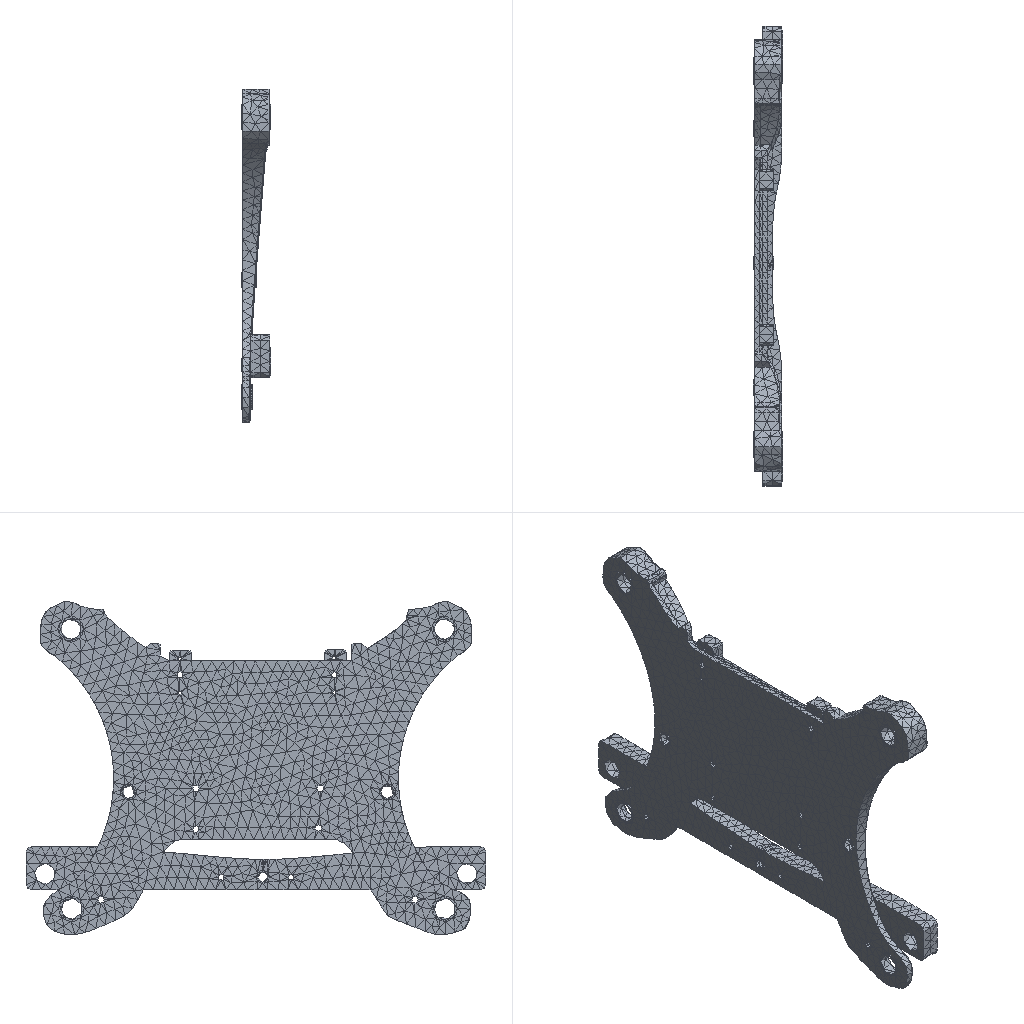Simulation study | ansys workbench
Ansys APDL input file, long lists of numbers shortened:
/batch
/config,noeldb,1     ! force off writing results to database
*get,_wallstrt,active,,time,wall
! ANSYS input file written by Workbench version 2022 R2
! File used for geometry attach:
/title,_____1--____ (A5)
! ****** Begin Custom Load Command Snippet ******
/COM, ACT Extensions:
/COM,     LSDYNA, 2022.2
/COM,/COM,     ANSYSMotion, 2022.2
/COM,
! ****** End   Custom Load Command Snippet ******
*DIM,_wb_ProjectScratch_dir,string,248
_wb_ProjectScratch_dir(1) = ''
*DIM,_wb_SolverFiles_dir,string,248
_wb_SolverFiles_dir(1) = ''
*DIM,_wb_userfiles_dir,string,248
_wb_userfiles_dir(1) = ''
/com,--- Data in consistent NMM units. See Solving Units in the help system for more information.
/units,MPA
/nopr
/wb,file,start              !  signify a WB generated input file
/prep7
! Turn off shape checking because checks already performed inside WB mesher.
! See help system for more information.
SHPP,OFF,,NOWARN
/nolist
etcon,set             ! allow ANSYS to choose best KEYOP's for 180x elements, resets any applicable keyopt to MAPDL defaults
/com,*********** Nodes for the whole assembly ***********
nblock,3,,33969
(1i9,3e20.9e3)
        1     3.263410559E+01     3.933549495E+02    -1.201904341E+02
! (30880 more lines like these left out)
-1
/wb,elem,start            !  set before creation of elements
/com,*********** Elements for Body 1 "_____(2)-FreeParts|_____(2)" ***********
et,1,187
eblock,19,solid,,16207
(19i9)
        1        1        1        1        0        0        0        0       10        0        1      141     2428     2638     4977     6172    21111     6173     6178
! (32413 more lines like these left out)
-1
/wb,elem,end               !  done creating elements
/com,*********** Send User Defined Coordinate System(s) ***********
csys,0
toffst,273.15,  ! Temperature offset from absolute zero
/com,*********** Set Reference Temperature ***********
tref,22.
/wb,mat,start              !  starting to send materials
/com,*********** Send Materials ***********
MP,DENS,1,7.85e-09,	! tonne mm^-3
MP,EX,1,210000,	! tonne s^-2 mm^-1
MP,NUXY,1,0.3,
/wb,mat,end                !  done sending materials
!************************* Model Summary ********************
!_____(2)-FreeParts|_____(2),	热扎酸洗高强度钢,	matid,	1
!************************* End Model Summary ********************
! get the diagonal of the bounding box. Needed later for other things
*get,_xmin,node,,mnloc,x
*get,_ymin,node,,mnloc,y
*get,_zmin,node,,mnloc,z
*get,_xmax,node,,mxloc,x
*get,_ymax,node,,mxloc,y
*get,_zmax,node,,mxloc,z
_ASMDIAG=(_xmax-_xmin)*(_xmax-_xmin)+(_ymax-_ymin)*(_ymax-_ymin)+(_zmax-_zmin)*(_zmax-_zmin)
_ASMDIAG=SQRT(_ASMDIAG)
/wb,contact,start          !  starting to send contact
/wb,contact,end            !  done creating contacts
/golist
/wb,load,start             !  starting to send loads
CMBLOCK,_CM34_FIXEDSU,NODE,      341
(8i10)
      2177      2178      2179      2180      2181      2182      2183      2192
! (42 more lines like these left out)
/com,*********** Fixed Supports ***********
CMBLOCK,_FIXEDSU,NODE,      341
(8i10)
      2177      2178      2179      2180      2181      2182      2183      2192
! (42 more lines like these left out)
cmsel,s,_FIXEDSU
d,all,all
nsel,all
/com,*********** Define Force Using Surface Effect Elements ***********
local,12,0,0.,0.,0.,0.,0.,0.
csys,0
et,2,154
eblock,10,,,88
(15i9)
    25038        2        2        2       12     2178     2179     4045     4045    20070    20078     4045    20073
! (87 more lines like these left out)
-1
esel,s,type,,2
keyop,2,2,1                ! Apply load in local coordinate system
keyop,2,7,1                ! Use original area so load is constant in large deformation
esel,all
/gst,on,on
fini
*get,_numnode,node,0,count
*get,_numelem,elem,0,count
*get, _MAXELEMNUM, elem, 0, NUM, MAX
*get, _MAXNODENUM, node, 0, NUM, MAX
*get, _MAXELEMTYPE, etyp, 0, NUM, MAX
*get, _MAXREALCONST, rcon, 0, NUM, MAX
/go
/wb,load,end               !  done creating loads
/com,--- Number of total nodes = %_numnode%
/com,--- Number of contact elements = 88
/com,--- Number of spring elements = 0
/com,--- Number of bearing elements = 0
/com,--- Number of solid elements = 16207
/com,--- Number of condensed parts = 0
/com,--- Number of total elements = %_numelem%
*get,_wallbsol,active,,time,wall
/com,****************************************************************************
/com,*************************    SOLUTION       ********************************
/com,****************************************************************************
/solu
antype,0                   ! static analysis
_thickRatio=  1     ! Ratio of thick parts in the model
eqsl,pcg,1e-8,,,,,,1
cntr,print,1               ! print out contact info and also make no initial contact an error
nldiag,cont,iter           ! print out contact info each equilibrium iteration
rescontrol,linear,last           ! Turn on restart files due to future eigen analysis intent
/com,****************************************************
/com,******************* SOLVE FOR LS 1 OF 1 ****************
esel,s,type,,2
nsle
sfe,all,1,pres,1,0.105
sfe,all,2,pres,1,0.
sfe,all,3,pres,1,0.
nsel,all
esel,all
acel,29430.,0.,0.
/nopr
/gopr
nsub,1,1,1
time,1.
outres,erase
outres,all,none
outres,nsol,all,
outres,rsol,all
outres,eangl,all
outres,etmp,all
outres,veng,all
outres,strs,all,
outres,epel,all,
outres,eppl,all,
outres,cont,all,
! *********** WB SOLVE COMMAND ***********
! check interactive state
*get,ANSINTER_,active,,int
*if,ANSINTER_,ne,0,then
/eof
*endif
solve
/com *************** Write FE CONNECTORS *********
CEWRITE,file,ce,,INTE
/com,****************************************************
/com,*************** FINISHED SOLVE FOR LS 1 *************
*get,_wallasol,active,,time,wall
/nopr
*get,_numnode,node,0,count
*get,_numelem,elem,0,count
*get, _MAXELEMNUM, elem, 0, NUM, MAX
*get, _MAXNODENUM, node, 0, NUM, MAX,,,INTERNAL
*get, _MAXELEMTYPE, etyp, 0, NUM, MAX
*get, _MAXREALCONST, rcon, 0, NUM, MAX
*get,_NSOLTHREADS,active,0,ntfs
*get,_NSOLPROCESSES,active,0,npfs
/gopr
*get,_PCGITER,active,,solu,cgiter
/post1
xmlo,ENCODING,ISO-8859-1
xmlo,parm
/xml,parm,xml
fini
/gopr
*get,_walldone,active,,time,wall
_preptime=(_wallbsol-_wallstrt)*3600
_solvtime=(_wallasol-_wallbsol)*3600
_posttime=(_walldone-_wallasol)*3600
_totaltim=(_walldone-_wallstrt)*3600
*get,_dlbratio,active,0,solu,dlbr
*get,_combtime,active,0,solu,comb
*get,_ssmode,active,0,solu,ssmm
*get,_ndofs,active,0,solu,ndof
/com,--- Total number of nodes = %_numnode%
/com,--- Total number of elements = %_numelem%
/com,--- Element load balance ratio = %_dlbratio%
/com,--- Time to combine distributed files = %_combtime%
/com,--- Sparse memory mode = %_ssmode%
/com,--- Number of DOF = %_ndofs%
/wb,file,end               ! done with WB generated input